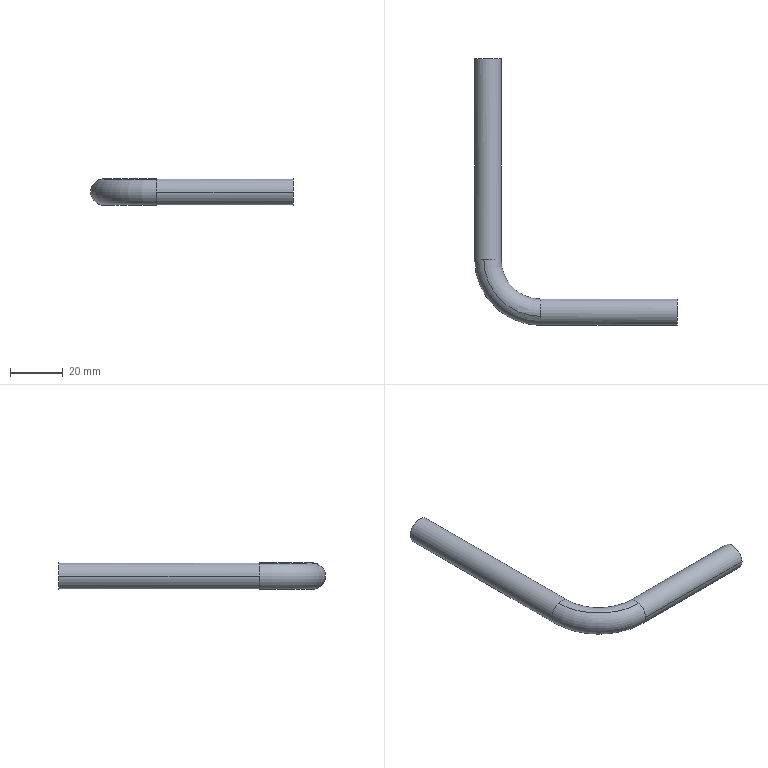Part | 1 solid | 8 faces | box 76.634 x 101 x 10 mm | volume 12492 mm3 | cylinder 4 | plane 2 | torus 2 | commonest cylinder face diameters 10 x4
STEP:
#1=CARTESIAN_POINT('',(0.,0.,0.));
#2=DIRECTION('',(0.,0.,1.));
#3=DIRECTION('',(1.,0.,0.));
#4=AXIS2_PLACEMENT_3D('',#1,#2,#3);
#5=CARTESIAN_POINT('',(-70.758,271.551,-68.051));
#6=VERTEX_POINT('',#5);
#7=CARTESIAN_POINT('',(-70.758,347.551,-68.051));
#8=VERTEX_POINT('',#7);
#9=CARTESIAN_POINT('',(-70.758,271.551,-68.051));
#10=DIRECTION('',(0.,1.,0.));
#11=VECTOR('',#10,1.);
#12=LINE('',#9,#11);
#13=CARTESIAN_POINT('',(-75.758,301.551,-68.051));
#14=DIRECTION('',(0.,1.,0.));
#15=DIRECTION('',(0.,0.,1.));
#16=AXIS2_PLACEMENT_3D('',#13,#14,#15);
#17=CYLINDRICAL_SURFACE('',#16,5.);
#18=CARTESIAN_POINT('',(1.571,-30.));
#19=DIRECTION('',(0.,1.));
#20=VECTOR('',#19,1.);
#21=LINE('',#18,#20);
#22=(GEOMETRIC_REPRESENTATION_CONTEXT(2)PARAMETRIC_REPRESENTATION_CONTEXT()REPRESENTATION_CONTEXT('',''));
#23=DEFINITIONAL_REPRESENTATION('',(#21),#22);
#24=PCURVE('',#17,#23);
#25=CARTESIAN_POINT('',(-75.758,301.551,-68.051));
#26=DIRECTION('',(0.,1.,0.));
#27=DIRECTION('',(0.,0.,-1.));
#28=AXIS2_PLACEMENT_3D('',#25,#26,#27);
#29=CYLINDRICAL_SURFACE('',#28,5.);
#30=CARTESIAN_POINT('',(4.712,-30.));
#31=DIRECTION('',(0.,1.));
#32=VECTOR('',#31,1.);
#33=LINE('',#30,#32);
#34=(GEOMETRIC_REPRESENTATION_CONTEXT(2)PARAMETRIC_REPRESENTATION_CONTEXT()REPRESENTATION_CONTEXT('',''));
#35=DEFINITIONAL_REPRESENTATION('',(#33),#34);
#36=PCURVE('',#29,#35);
#37=SURFACE_CURVE('',#12,(#24,#36),.PCURVE_S1.);
#38=EDGE_CURVE('',#6,#8,#37,.T.);
#39=ORIENTED_EDGE('',*,*,#38,.F.);
#40=CARTESIAN_POINT('',(-74.213,271.551,-72.807));
#41=VERTEX_POINT('',#40);
#42=CARTESIAN_POINT('',(-75.758,271.551,-68.051));
#43=DIRECTION('',(0.,1.,0.));
#44=DIRECTION('',(-1.,0.,0.));
#45=AXIS2_PLACEMENT_3D('',#42,#43,#44);
#46=CIRCLE('',#45,5.);
#47=CARTESIAN_POINT('',(-1.571,-30.));
#48=DIRECTION('',(1.,0.));
#49=VECTOR('',#48,1.);
#50=LINE('',#47,#49);
#51=(GEOMETRIC_REPRESENTATION_CONTEXT(2)PARAMETRIC_REPRESENTATION_CONTEXT()REPRESENTATION_CONTEXT('',''));
#52=DEFINITIONAL_REPRESENTATION('',(#50),#51);
#53=PCURVE('',#17,#52);
#54=CARTESIAN_POINT('',(-55.758,271.551,-68.051));
#55=DIRECTION('',(0.,0.,1.));
#56=DIRECTION('',(0.7071,0.7071,0.));
#57=AXIS2_PLACEMENT_3D('',#54,#55,#56);
#58=TOROIDAL_SURFACE('',#57,20.,5.);
#59=CARTESIAN_POINT('',(2.356,0.));
#60=DIRECTION('',(0.,1.));
#61=VECTOR('',#60,1.);
#62=LINE('',#59,#61);
#63=(GEOMETRIC_REPRESENTATION_CONTEXT(2)PARAMETRIC_REPRESENTATION_CONTEXT()REPRESENTATION_CONTEXT('',''));
#64=DEFINITIONAL_REPRESENTATION('',(#62),#63);
#65=PCURVE('',#58,#64);
#66=SURFACE_CURVE('',#46,(#53,#65),.PCURVE_S1.);
#67=EDGE_CURVE('',#6,#41,#66,.T.);
#68=ORIENTED_EDGE('',*,*,#67,.T.);
#69=CARTESIAN_POINT('',(-80.758,271.551,-68.051));
#70=VERTEX_POINT('',#69);
#71=CARTESIAN_POINT('',(-75.758,271.551,-68.051));
#72=DIRECTION('',(0.,1.,0.));
#73=DIRECTION('',(-1.,0.,0.));
#74=AXIS2_PLACEMENT_3D('',#71,#72,#73);
#75=CIRCLE('',#74,5.);
#76=CARTESIAN_POINT('',(-1.571,-30.));
#77=DIRECTION('',(1.,0.));
#78=VECTOR('',#77,1.);
#79=LINE('',#76,#78);
#80=(GEOMETRIC_REPRESENTATION_CONTEXT(2)PARAMETRIC_REPRESENTATION_CONTEXT()REPRESENTATION_CONTEXT('',''));
#81=DEFINITIONAL_REPRESENTATION('',(#79),#80);
#82=PCURVE('',#17,#81);
#83=CARTESIAN_POINT('',(-55.758,271.551,-68.051));
#84=DIRECTION('',(0.,0.,1.));
#85=DIRECTION('',(0.7071,0.7071,0.));
#86=AXIS2_PLACEMENT_3D('',#83,#84,#85);
#87=TOROIDAL_SURFACE('',#86,20.,5.);
#88=CARTESIAN_POINT('',(2.356,0.));
#89=DIRECTION('',(0.,1.));
#90=VECTOR('',#89,1.);
#91=LINE('',#88,#90);
#92=(GEOMETRIC_REPRESENTATION_CONTEXT(2)PARAMETRIC_REPRESENTATION_CONTEXT()REPRESENTATION_CONTEXT('',''));
#93=DEFINITIONAL_REPRESENTATION('',(#91),#92);
#94=PCURVE('',#87,#93);
#95=SURFACE_CURVE('',#75,(#82,#94),.PCURVE_S1.);
#96=EDGE_CURVE('',#41,#70,#95,.T.);
#97=ORIENTED_EDGE('',*,*,#96,.T.);
#98=CARTESIAN_POINT('',(-80.758,347.551,-68.051));
#99=VERTEX_POINT('',#98);
#100=CARTESIAN_POINT('',(-80.758,271.551,-68.051));
#101=DIRECTION('',(0.,1.,0.));
#102=VECTOR('',#101,1.);
#103=LINE('',#100,#102);
#104=CARTESIAN_POINT('',(4.712,-30.));
#105=DIRECTION('',(0.,1.));
#106=VECTOR('',#105,1.);
#107=LINE('',#104,#106);
#108=(GEOMETRIC_REPRESENTATION_CONTEXT(2)PARAMETRIC_REPRESENTATION_CONTEXT()REPRESENTATION_CONTEXT('',''));
#109=DEFINITIONAL_REPRESENTATION('',(#107),#108);
#110=PCURVE('',#17,#109);
#111=CARTESIAN_POINT('',(1.571,-30.));
#112=DIRECTION('',(0.,1.));
#113=VECTOR('',#112,1.);
#114=LINE('',#111,#113);
#115=(GEOMETRIC_REPRESENTATION_CONTEXT(2)PARAMETRIC_REPRESENTATION_CONTEXT()REPRESENTATION_CONTEXT('',''));
#116=DEFINITIONAL_REPRESENTATION('',(#114),#115);
#117=PCURVE('',#29,#116);
#118=SURFACE_CURVE('',#103,(#110,#117),.PCURVE_S1.);
#119=EDGE_CURVE('',#70,#99,#118,.T.);
#120=ORIENTED_EDGE('',*,*,#119,.T.);
#121=CARTESIAN_POINT('',(-75.758,347.551,-68.051));
#122=DIRECTION('',(0.,1.,0.));
#123=DIRECTION('',(-1.,0.,0.));
#124=AXIS2_PLACEMENT_3D('',#121,#122,#123);
#125=CIRCLE('',#124,5.);
#126=CARTESIAN_POINT('',(-1.571,46.));
#127=DIRECTION('',(1.,0.));
#128=VECTOR('',#127,1.);
#129=LINE('',#126,#128);
#130=(GEOMETRIC_REPRESENTATION_CONTEXT(2)PARAMETRIC_REPRESENTATION_CONTEXT()REPRESENTATION_CONTEXT('',''));
#131=DEFINITIONAL_REPRESENTATION('',(#129),#130);
#132=PCURVE('',#17,#131);
#133=CARTESIAN_POINT('',(-75.758,347.551,-68.051));
#134=DIRECTION('',(0.,1.,0.));
#135=DIRECTION('',(-1.,0.,0.));
#136=AXIS2_PLACEMENT_3D('',#133,#134,#135);
#137=PLANE('',#136);
#138=CARTESIAN_POINT('',(0.,0.));
#139=DIRECTION('',(1.,0.));
#140=AXIS2_PLACEMENT_2D('',#138,#139);
#141=CIRCLE('',#140,5.);
#142=(GEOMETRIC_REPRESENTATION_CONTEXT(2)PARAMETRIC_REPRESENTATION_CONTEXT()REPRESENTATION_CONTEXT('',''));
#143=DEFINITIONAL_REPRESENTATION('',(#141),#142);
#144=PCURVE('',#137,#143);
#145=SURFACE_CURVE('',#125,(#132,#144),.PCURVE_S1.);
#146=EDGE_CURVE('',#8,#99,#145,.T.);
#147=ORIENTED_EDGE('',*,*,#146,.F.);
#148=EDGE_LOOP('',(#39,#68,#97,#120,#147));
#149=FACE_BOUND('',#148,.T.);
#150=ADVANCED_FACE('',(#149),#17,.T.);
#151=CARTESIAN_POINT('',(-75.758,347.551,-68.051));
#152=DIRECTION('',(0.,1.,0.));
#153=DIRECTION('',(-1.,0.,0.));
#154=AXIS2_PLACEMENT_3D('',#151,#152,#153);
#155=CIRCLE('',#154,5.);
#156=CARTESIAN_POINT('',(0.,0.));
#157=DIRECTION('',(1.,0.));
#158=AXIS2_PLACEMENT_2D('',#156,#157);
#159=CIRCLE('',#158,5.);
#160=(GEOMETRIC_REPRESENTATION_CONTEXT(2)PARAMETRIC_REPRESENTATION_CONTEXT()REPRESENTATION_CONTEXT('',''));
#161=DEFINITIONAL_REPRESENTATION('',(#159),#160);
#162=PCURVE('',#137,#161);
#163=CARTESIAN_POINT('',(1.571,46.));
#164=DIRECTION('',(1.,0.));
#165=VECTOR('',#164,1.);
#166=LINE('',#163,#165);
#167=(GEOMETRIC_REPRESENTATION_CONTEXT(2)PARAMETRIC_REPRESENTATION_CONTEXT()REPRESENTATION_CONTEXT('',''));
#168=DEFINITIONAL_REPRESENTATION('',(#166),#167);
#169=PCURVE('',#29,#168);
#170=SURFACE_CURVE('',#155,(#162,#169),.PCURVE_S1.);
#171=EDGE_CURVE('',#99,#8,#170,.T.);
#172=ORIENTED_EDGE('',*,*,#171,.T.);
#173=ORIENTED_EDGE('',*,*,#146,.T.);
#174=EDGE_LOOP('',(#172,#173));
#175=FACE_BOUND('',#174,.T.);
#176=ADVANCED_FACE('',(#175),#137,.T.);
#177=CARTESIAN_POINT('',(-55.758,253.096,-72.807));
#178=VERTEX_POINT('',#177);
#179=CARTESIAN_POINT('',(-55.758,271.551,-72.807));
#180=DIRECTION('',(0.,0.,1.));
#181=DIRECTION('',(-1.,0.,0.));
#182=AXIS2_PLACEMENT_3D('',#179,#180,#181);
#183=CIRCLE('',#182,18.455);
#184=CARTESIAN_POINT('',(2.356,4.398));
#185=DIRECTION('',(1.,0.));
#186=VECTOR('',#185,1.);
#187=LINE('',#184,#186);
#188=(GEOMETRIC_REPRESENTATION_CONTEXT(2)PARAMETRIC_REPRESENTATION_CONTEXT()REPRESENTATION_CONTEXT('',''));
#189=DEFINITIONAL_REPRESENTATION('',(#187),#188);
#190=PCURVE('',#58,#189);
#191=CARTESIAN_POINT('',(2.356,4.398));
#192=DIRECTION('',(1.,0.));
#193=VECTOR('',#192,1.);
#194=LINE('',#191,#193);
#195=(GEOMETRIC_REPRESENTATION_CONTEXT(2)PARAMETRIC_REPRESENTATION_CONTEXT()REPRESENTATION_CONTEXT('',''));
#196=DEFINITIONAL_REPRESENTATION('',(#194),#195);
#197=PCURVE('',#87,#196);
#198=SURFACE_CURVE('',#183,(#190,#197),.PCURVE_S1.);
#199=EDGE_CURVE('',#41,#178,#198,.T.);
#200=ORIENTED_EDGE('',*,*,#199,.F.);
#201=ORIENTED_EDGE('',*,*,#67,.F.);
#202=CARTESIAN_POINT('',(-77.304,271.551,-63.296));
#203=VERTEX_POINT('',#202);
#204=CARTESIAN_POINT('',(-75.758,271.551,-68.051));
#205=DIRECTION('',(0.,1.,0.));
#206=DIRECTION('',(-1.,0.,0.));
#207=AXIS2_PLACEMENT_3D('',#204,#205,#206);
#208=CIRCLE('',#207,5.);
#209=CARTESIAN_POINT('',(2.356,0.));
#210=DIRECTION('',(0.,1.));
#211=VECTOR('',#210,1.);
#212=LINE('',#209,#211);
#213=(GEOMETRIC_REPRESENTATION_CONTEXT(2)PARAMETRIC_REPRESENTATION_CONTEXT()REPRESENTATION_CONTEXT('',''));
#214=DEFINITIONAL_REPRESENTATION('',(#212),#213);
#215=PCURVE('',#58,#214);
#216=CARTESIAN_POINT('',(1.571,-30.));
#217=DIRECTION('',(1.,0.));
#218=VECTOR('',#217,1.);
#219=LINE('',#216,#218);
#220=(GEOMETRIC_REPRESENTATION_CONTEXT(2)PARAMETRIC_REPRESENTATION_CONTEXT()REPRESENTATION_CONTEXT('',''));
#221=DEFINITIONAL_REPRESENTATION('',(#219),#220);
#222=PCURVE('',#29,#221);
#223=SURFACE_CURVE('',#208,(#215,#222),.PCURVE_S1.);
#224=EDGE_CURVE('',#203,#6,#223,.T.);
#225=ORIENTED_EDGE('',*,*,#224,.F.);
#226=CARTESIAN_POINT('',(-55.758,250.006,-63.296));
#227=VERTEX_POINT('',#226);
#228=CARTESIAN_POINT('',(-55.758,271.551,-63.296));
#229=DIRECTION('',(0.,0.,1.));
#230=DIRECTION('',(-1.,0.,0.));
#231=AXIS2_PLACEMENT_3D('',#228,#229,#230);
#232=CIRCLE('',#231,21.545);
#233=CARTESIAN_POINT('',(2.356,1.257));
#234=DIRECTION('',(1.,0.));
#235=VECTOR('',#234,1.);
#236=LINE('',#233,#235);
#237=(GEOMETRIC_REPRESENTATION_CONTEXT(2)PARAMETRIC_REPRESENTATION_CONTEXT()REPRESENTATION_CONTEXT('',''));
#238=DEFINITIONAL_REPRESENTATION('',(#236),#237);
#239=PCURVE('',#58,#238);
#240=CARTESIAN_POINT('',(2.356,7.54));
#241=DIRECTION('',(1.,0.));
#242=VECTOR('',#241,1.);
#243=LINE('',#240,#242);
#244=(GEOMETRIC_REPRESENTATION_CONTEXT(2)PARAMETRIC_REPRESENTATION_CONTEXT()REPRESENTATION_CONTEXT('',''));
#245=DEFINITIONAL_REPRESENTATION('',(#243),#244);
#246=PCURVE('',#87,#245);
#247=SURFACE_CURVE('',#232,(#239,#246),.PCURVE_S1.);
#248=EDGE_CURVE('',#203,#227,#247,.T.);
#249=ORIENTED_EDGE('',*,*,#248,.T.);
#250=CARTESIAN_POINT('',(-55.758,256.551,-68.051));
#251=VERTEX_POINT('',#250);
#252=CARTESIAN_POINT('',(-55.758,251.551,-68.051));
#253=DIRECTION('',(-1.,0.,0.));
#254=DIRECTION('',(0.,-1.,0.));
#255=AXIS2_PLACEMENT_3D('',#252,#253,#254);
#256=CIRCLE('',#255,5.);
#257=CARTESIAN_POINT('',(3.927,0.));
#258=DIRECTION('',(0.,1.));
#259=VECTOR('',#258,1.);
#260=LINE('',#257,#259);
#261=(GEOMETRIC_REPRESENTATION_CONTEXT(2)PARAMETRIC_REPRESENTATION_CONTEXT()REPRESENTATION_CONTEXT('',''));
#262=DEFINITIONAL_REPRESENTATION('',(#260),#261);
#263=PCURVE('',#58,#262);
#264=CARTESIAN_POINT('',(-55.758,251.551,-68.051));
#265=DIRECTION('',(1.,0.,0.));
#266=DIRECTION('',(0.,0.,-1.));
#267=AXIS2_PLACEMENT_3D('',#264,#265,#266);
#268=CYLINDRICAL_SURFACE('',#267,5.);
#269=CARTESIAN_POINT('',(4.712,0.));
#270=DIRECTION('',(-1.,0.));
#271=VECTOR('',#270,1.);
#272=LINE('',#269,#271);
#273=(GEOMETRIC_REPRESENTATION_CONTEXT(2)PARAMETRIC_REPRESENTATION_CONTEXT()REPRESENTATION_CONTEXT('',''));
#274=DEFINITIONAL_REPRESENTATION('',(#272),#273);
#275=PCURVE('',#268,#274);
#276=SURFACE_CURVE('',#256,(#263,#275),.PCURVE_S1.);
#277=EDGE_CURVE('',#227,#251,#276,.T.);
#278=ORIENTED_EDGE('',*,*,#277,.T.);
#279=CARTESIAN_POINT('',(-55.758,251.551,-68.051));
#280=DIRECTION('',(-1.,0.,0.));
#281=DIRECTION('',(0.,-1.,0.));
#282=AXIS2_PLACEMENT_3D('',#279,#280,#281);
#283=CIRCLE('',#282,5.);
#284=CARTESIAN_POINT('',(3.927,0.));
#285=DIRECTION('',(0.,1.));
#286=VECTOR('',#285,1.);
#287=LINE('',#284,#286);
#288=(GEOMETRIC_REPRESENTATION_CONTEXT(2)PARAMETRIC_REPRESENTATION_CONTEXT()REPRESENTATION_CONTEXT('',''));
#289=DEFINITIONAL_REPRESENTATION('',(#287),#288);
#290=PCURVE('',#58,#289);
#291=CARTESIAN_POINT('',(-55.758,251.551,-68.051));
#292=DIRECTION('',(1.,0.,0.));
#293=DIRECTION('',(0.,0.,1.));
#294=AXIS2_PLACEMENT_3D('',#291,#292,#293);
#295=CYLINDRICAL_SURFACE('',#294,5.);
#296=CARTESIAN_POINT('',(7.854,0.));
#297=DIRECTION('',(-1.,0.));
#298=VECTOR('',#297,1.);
#299=LINE('',#296,#298);
#300=(GEOMETRIC_REPRESENTATION_CONTEXT(2)PARAMETRIC_REPRESENTATION_CONTEXT()REPRESENTATION_CONTEXT('',''));
#301=DEFINITIONAL_REPRESENTATION('',(#299),#300);
#302=PCURVE('',#295,#301);
#303=SURFACE_CURVE('',#283,(#290,#302),.PCURVE_S1.);
#304=EDGE_CURVE('',#251,#178,#303,.T.);
#305=ORIENTED_EDGE('',*,*,#304,.T.);
#306=EDGE_LOOP('',(#200,#201,#225,#249,#278,#305));
#307=FACE_BOUND('',#306,.T.);
#308=ADVANCED_FACE('',(#307),#58,.T.);
#309=CARTESIAN_POINT('',(-55.758,246.551,-68.051));
#310=VERTEX_POINT('',#309);
#311=CARTESIAN_POINT('',(-4.124,246.551,-68.051));
#312=VERTEX_POINT('',#311);
#313=CARTESIAN_POINT('',(-55.758,246.551,-68.051));
#314=DIRECTION('',(1.,0.,0.));
#315=VECTOR('',#314,1.);
#316=LINE('',#313,#315);
#317=CARTESIAN_POINT('',(1.571,0.));
#318=DIRECTION('',(0.,1.));
#319=VECTOR('',#318,1.);
#320=LINE('',#317,#319);
#321=(GEOMETRIC_REPRESENTATION_CONTEXT(2)PARAMETRIC_REPRESENTATION_CONTEXT()REPRESENTATION_CONTEXT('',''));
#322=DEFINITIONAL_REPRESENTATION('',(#320),#321);
#323=PCURVE('',#295,#322);
#324=CARTESIAN_POINT('',(4.712,0.));
#325=DIRECTION('',(0.,1.));
#326=VECTOR('',#325,1.);
#327=LINE('',#324,#326);
#328=(GEOMETRIC_REPRESENTATION_CONTEXT(2)PARAMETRIC_REPRESENTATION_CONTEXT()REPRESENTATION_CONTEXT('',''));
#329=DEFINITIONAL_REPRESENTATION('',(#327),#328);
#330=PCURVE('',#268,#329);
#331=SURFACE_CURVE('',#316,(#323,#330),.PCURVE_S1.);
#332=EDGE_CURVE('',#310,#312,#331,.T.);
#333=ORIENTED_EDGE('',*,*,#332,.F.);
#334=CARTESIAN_POINT('',(-55.758,251.551,-68.051));
#335=DIRECTION('',(-1.,0.,0.));
#336=DIRECTION('',(0.,-1.,0.));
#337=AXIS2_PLACEMENT_3D('',#334,#335,#336);
#338=CIRCLE('',#337,5.);
#339=CARTESIAN_POINT('',(7.854,0.));
#340=DIRECTION('',(-1.,0.));
#341=VECTOR('',#340,1.);
#342=LINE('',#339,#341);
#343=(GEOMETRIC_REPRESENTATION_CONTEXT(2)PARAMETRIC_REPRESENTATION_CONTEXT()REPRESENTATION_CONTEXT('',''));
#344=DEFINITIONAL_REPRESENTATION('',(#342),#343);
#345=PCURVE('',#295,#344);
#346=CARTESIAN_POINT('',(3.927,0.));
#347=DIRECTION('',(0.,1.));
#348=VECTOR('',#347,1.);
#349=LINE('',#346,#348);
#350=(GEOMETRIC_REPRESENTATION_CONTEXT(2)PARAMETRIC_REPRESENTATION_CONTEXT()REPRESENTATION_CONTEXT('',''));
#351=DEFINITIONAL_REPRESENTATION('',(#349),#350);
#352=PCURVE('',#87,#351);
#353=SURFACE_CURVE('',#338,(#345,#352),.PCURVE_S1.);
#354=EDGE_CURVE('',#178,#310,#353,.T.);
#355=ORIENTED_EDGE('',*,*,#354,.F.);
#356=ORIENTED_EDGE('',*,*,#304,.F.);
#357=CARTESIAN_POINT('',(-4.124,256.551,-68.051));
#358=VERTEX_POINT('',#357);
#359=CARTESIAN_POINT('',(-55.758,256.551,-68.051));
#360=DIRECTION('',(1.,0.,0.));
#361=VECTOR('',#360,1.);
#362=LINE('',#359,#361);
#363=CARTESIAN_POINT('',(4.712,0.));
#364=DIRECTION('',(0.,1.));
#365=VECTOR('',#364,1.);
#366=LINE('',#363,#365);
#367=(GEOMETRIC_REPRESENTATION_CONTEXT(2)PARAMETRIC_REPRESENTATION_CONTEXT()REPRESENTATION_CONTEXT('',''));
#368=DEFINITIONAL_REPRESENTATION('',(#366),#367);
#369=PCURVE('',#295,#368);
#370=CARTESIAN_POINT('',(1.571,0.));
#371=DIRECTION('',(0.,1.));
#372=VECTOR('',#371,1.);
#373=LINE('',#370,#372);
#374=(GEOMETRIC_REPRESENTATION_CONTEXT(2)PARAMETRIC_REPRESENTATION_CONTEXT()REPRESENTATION_CONTEXT('',''));
#375=DEFINITIONAL_REPRESENTATION('',(#373),#374);
#376=PCURVE('',#268,#375);
#377=SURFACE_CURVE('',#362,(#369,#376),.PCURVE_S1.);
#378=EDGE_CURVE('',#251,#358,#377,.T.);
#379=ORIENTED_EDGE('',*,*,#378,.T.);
#380=CARTESIAN_POINT('',(-4.124,251.551,-68.051));
#381=DIRECTION('',(-1.,0.,0.));
#382=DIRECTION('',(0.,1.,0.));
#383=AXIS2_PLACEMENT_3D('',#380,#381,#382);
#384=CIRCLE('',#383,5.);
#385=CARTESIAN_POINT('',(4.712,51.634));
#386=DIRECTION('',(-1.,0.));
#387=VECTOR('',#386,1.);
#388=LINE('',#385,#387);
#389=(GEOMETRIC_REPRESENTATION_CONTEXT(2)PARAMETRIC_REPRESENTATION_CONTEXT()REPRESENTATION_CONTEXT('',''));
#390=DEFINITIONAL_REPRESENTATION('',(#388),#389);
#391=PCURVE('',#295,#390);
#392=CARTESIAN_POINT('',(-4.124,251.551,-68.051));
#393=DIRECTION('',(-1.,0.,0.));
#394=DIRECTION('',(0.,-1.,0.));
#395=AXIS2_PLACEMENT_3D('',#392,#393,#394);
#396=PLANE('',#395);
#397=CARTESIAN_POINT('',(0.,0.));
#398=DIRECTION('',(-1.,0.));
#399=AXIS2_PLACEMENT_2D('',#397,#398);
#400=CIRCLE('',#399,5.);
#401=(GEOMETRIC_REPRESENTATION_CONTEXT(2)PARAMETRIC_REPRESENTATION_CONTEXT()REPRESENTATION_CONTEXT('',''));
#402=DEFINITIONAL_REPRESENTATION('',(#400),#401);
#403=PCURVE('',#396,#402);
#404=SURFACE_CURVE('',#384,(#391,#403),.PCURVE_S1.);
#405=EDGE_CURVE('',#358,#312,#404,.T.);
#406=ORIENTED_EDGE('',*,*,#405,.T.);
#407=EDGE_LOOP('',(#333,#355,#356,#379,#406));
#408=FACE_BOUND('',#407,.T.);
#409=ADVANCED_FACE('',(#408),#295,.T.);
#410=CARTESIAN_POINT('',(-4.124,251.551,-68.051));
#411=DIRECTION('',(-1.,0.,0.));
#412=DIRECTION('',(0.,1.,0.));
#413=AXIS2_PLACEMENT_3D('',#410,#411,#412);
#414=CIRCLE('',#413,5.);
#415=CARTESIAN_POINT('',(0.,0.));
#416=DIRECTION('',(-1.,0.));
#417=AXIS2_PLACEMENT_2D('',#415,#416);
#418=CIRCLE('',#417,5.);
#419=(GEOMETRIC_REPRESENTATION_CONTEXT(2)PARAMETRIC_REPRESENTATION_CONTEXT()REPRESENTATION_CONTEXT('',''));
#420=DEFINITIONAL_REPRESENTATION('',(#418),#419);
#421=PCURVE('',#396,#420);
#422=CARTESIAN_POINT('',(7.854,51.634));
#423=DIRECTION('',(-1.,0.));
#424=VECTOR('',#423,1.);
#425=LINE('',#422,#424);
#426=(GEOMETRIC_REPRESENTATION_CONTEXT(2)PARAMETRIC_REPRESENTATION_CONTEXT()REPRESENTATION_CONTEXT('',''));
#427=DEFINITIONAL_REPRESENTATION('',(#425),#426);
#428=PCURVE('',#268,#427);
#429=SURFACE_CURVE('',#414,(#421,#428),.PCURVE_S1.);
#430=EDGE_CURVE('',#312,#358,#429,.T.);
#431=ORIENTED_EDGE('',*,*,#430,.F.);
#432=ORIENTED_EDGE('',*,*,#405,.F.);
#433=EDGE_LOOP('',(#431,#432));
#434=FACE_BOUND('',#433,.T.);
#435=ADVANCED_FACE('',(#434),#396,.F.);
#436=ORIENTED_EDGE('',*,*,#38,.T.);
#437=ORIENTED_EDGE('',*,*,#171,.F.);
#438=ORIENTED_EDGE('',*,*,#119,.F.);
#439=CARTESIAN_POINT('',(-75.758,271.551,-68.051));
#440=DIRECTION('',(0.,1.,0.));
#441=DIRECTION('',(-1.,0.,0.));
#442=AXIS2_PLACEMENT_3D('',#439,#440,#441);
#443=CIRCLE('',#442,5.);
#444=CARTESIAN_POINT('',(1.571,-30.));
#445=DIRECTION('',(1.,0.));
#446=VECTOR('',#445,1.);
#447=LINE('',#444,#446);
#448=(GEOMETRIC_REPRESENTATION_CONTEXT(2)PARAMETRIC_REPRESENTATION_CONTEXT()REPRESENTATION_CONTEXT('',''));
#449=DEFINITIONAL_REPRESENTATION('',(#447),#448);
#450=PCURVE('',#29,#449);
#451=CARTESIAN_POINT('',(2.356,6.283));
#452=DIRECTION('',(0.,1.));
#453=VECTOR('',#452,1.);
#454=LINE('',#451,#453);
#455=(GEOMETRIC_REPRESENTATION_CONTEXT(2)PARAMETRIC_REPRESENTATION_CONTEXT()REPRESENTATION_CONTEXT('',''));
#456=DEFINITIONAL_REPRESENTATION('',(#454),#455);
#457=PCURVE('',#87,#456);
#458=SURFACE_CURVE('',#443,(#450,#457),.PCURVE_S1.);
#459=EDGE_CURVE('',#70,#203,#458,.T.);
#460=ORIENTED_EDGE('',*,*,#459,.T.);
#461=ORIENTED_EDGE('',*,*,#224,.T.);
#462=EDGE_LOOP('',(#436,#437,#438,#460,#461));
#463=FACE_BOUND('',#462,.T.);
#464=ADVANCED_FACE('',(#463),#29,.T.);
#465=ORIENTED_EDGE('',*,*,#199,.T.);
#466=ORIENTED_EDGE('',*,*,#354,.T.);
#467=CARTESIAN_POINT('',(-55.758,251.551,-68.051));
#468=DIRECTION('',(-1.,0.,0.));
#469=DIRECTION('',(0.,-1.,0.));
#470=AXIS2_PLACEMENT_3D('',#467,#468,#469);
#471=CIRCLE('',#470,5.);
#472=CARTESIAN_POINT('',(3.927,6.283));
#473=DIRECTION('',(0.,1.));
#474=VECTOR('',#473,1.);
#475=LINE('',#472,#474);
#476=(GEOMETRIC_REPRESENTATION_CONTEXT(2)PARAMETRIC_REPRESENTATION_CONTEXT()REPRESENTATION_CONTEXT('',''));
#477=DEFINITIONAL_REPRESENTATION('',(#475),#476);
#478=PCURVE('',#87,#477);
#479=CARTESIAN_POINT('',(4.712,0.));
#480=DIRECTION('',(-1.,0.));
#481=VECTOR('',#480,1.);
#482=LINE('',#479,#481);
#483=(GEOMETRIC_REPRESENTATION_CONTEXT(2)PARAMETRIC_REPRESENTATION_CONTEXT()REPRESENTATION_CONTEXT('',''));
#484=DEFINITIONAL_REPRESENTATION('',(#482),#483);
#485=PCURVE('',#268,#484);
#486=SURFACE_CURVE('',#471,(#478,#485),.PCURVE_S1.);
#487=EDGE_CURVE('',#310,#227,#486,.T.);
#488=ORIENTED_EDGE('',*,*,#487,.T.);
#489=ORIENTED_EDGE('',*,*,#248,.F.);
#490=ORIENTED_EDGE('',*,*,#459,.F.);
#491=ORIENTED_EDGE('',*,*,#96,.F.);
#492=EDGE_LOOP('',(#465,#466,#488,#489,#490,#491));
#493=FACE_BOUND('',#492,.T.);
#494=ADVANCED_FACE('',(#493),#87,.T.);
#495=ORIENTED_EDGE('',*,*,#332,.T.);
#496=ORIENTED_EDGE('',*,*,#430,.T.);
#497=ORIENTED_EDGE('',*,*,#378,.F.);
#498=ORIENTED_EDGE('',*,*,#277,.F.);
#499=ORIENTED_EDGE('',*,*,#487,.F.);
#500=EDGE_LOOP('',(#495,#496,#497,#498,#499));
#501=FACE_BOUND('',#500,.T.);
#502=ADVANCED_FACE('',(#501),#268,.T.);
#503=CLOSED_SHELL('',(#150,#176,#308,#409,#435,#464,#494,#502));
#504=MANIFOLD_SOLID_BREP('',#503);
#505=(LENGTH_UNIT()NAMED_UNIT(*)SI_UNIT(.MILLI.,.METRE.));
#506=UNCERTAINTY_MEASURE_WITH_UNIT(LENGTH_MEASURE(0.0000001),#505,'','');
#507=(NAMED_UNIT(*)PLANE_ANGLE_UNIT()SI_UNIT($,.RADIAN.));
#508=(NAMED_UNIT(*)SI_UNIT($,.STERADIAN.)SOLID_ANGLE_UNIT());
#509=(GEOMETRIC_REPRESENTATION_CONTEXT(3)GLOBAL_UNCERTAINTY_ASSIGNED_CONTEXT((#506))GLOBAL_UNIT_ASSIGNED_CONTEXT((#505,#507,#508))REPRESENTATION_CONTEXT('',''));
#510=ADVANCED_BREP_SHAPE_REPRESENTATION('',(#4,#504),#509);